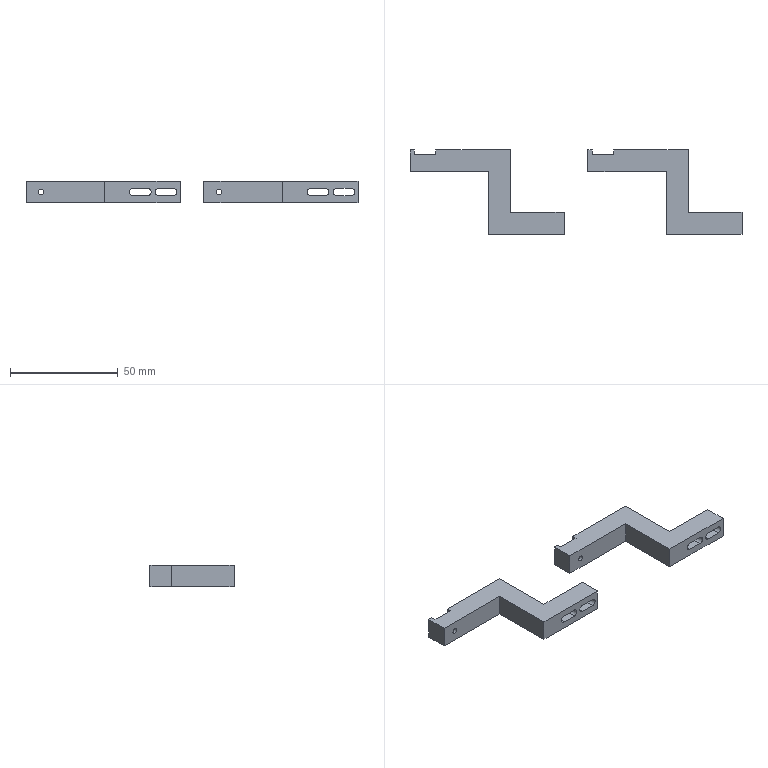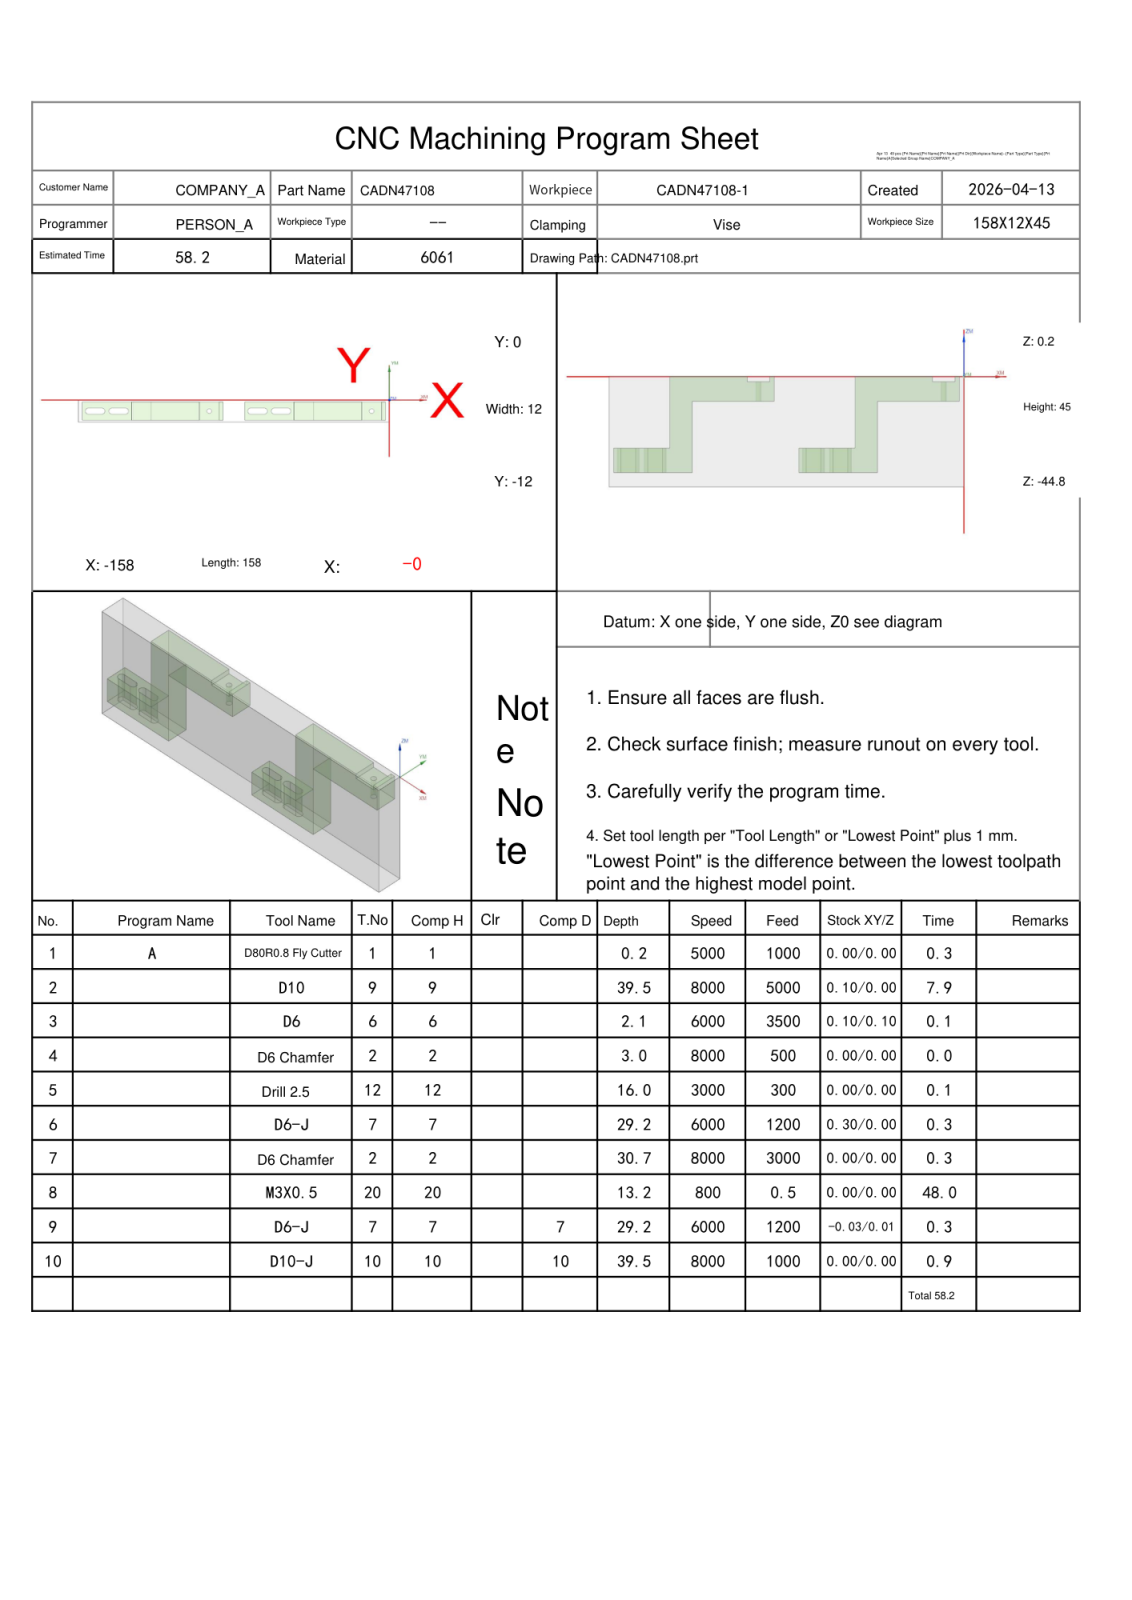NC program | NX | posted by the shop | part box 154 x 39 x 10 mm
Whole program, first 2157 of 3604 lines:
%
O0001
(Machine time: 104.10 MIN)
(===Total Tool:8===)
(T1=D80R0.8 Fly Cutter D=80.  R=0.8  D-  H01 Z=0.    )
(T9=D10     D=10.  R=0.   D-  H09 Z=-39.3 )
(T6=D6      D=6.   R=0.   D-  H06 Z=-1.9  )
(T2=D6 Chamfer   D=6.   R=0.   D-  H02 Z=-30.5 )
(T12=Drill 2.5  D=2.5  DR_a=118 D-  H12 Z=-15.75)
(T7=D6-J    D=6.   R=0.   D-  H07 Z=-29.  )
(T20=M3X0.5 D=2.5  DR_a=180 D-  H20 Z=-13.  )
(T10=D10-J  D=10.  R=0.   D10 H10 Z=-39.3 )
G80 G90 G17 G49 G40
G91 G28 Z0
M01
N1 T01 M06
(D80R0.8 Fly Cutter  D=80. R=0.8 H=01 ce=0.00 di=0.00)
G00 G90 G54 X-201. Y-6. M03 S5000
G43 H01 Z20.
M08
Z2.
G01 Z0.0 F1000.
X-196.
X38.
X43.
Z2.
G00 Z20.
G91 G28 Z0.0
M05
M09
G91 G28 Z0.0
M01
N2 T09 M06
(D10  D=10. R=0. H=09 ce=0.10 di=0.00)
G00 G90 G54 X-120.25 Y-16.1 M03 S8000
G43 H09 Z20.
M08
Z.5
G01 X-156. Z.354 F5000.
G02 X-161.1 Y-11. Z.321 I0.0 J5.1
G01 Y-1. Z.281
G02 X-156. Y4.1 Z.248 I5.1 J0.0
G01 X-84.5 Z-.044
G02 X-79.4 Y-1. Z-.077 I0.0 J-5.1
G01 Y-11. Z-.117
G02 X-84.5 Y-16.1 Z-.15 I-5.1 J0.0
G01 X-156. Z-.442
G02 X-161.1 Y-11. Z-.475 I0.0 J5.1
G01 Y-1. Z-.515
G02 X-156. Y4.1 Z-.548 I5.1 J0.0
G01 X-84.5 Z-.84
G02 X-79.4 Y-1. Z-.873 I0.0 J-5.1
G01 Y-11. Z-.913
G02 X-84.5 Y-16.1 Z-.946 I-5.1 J0.0
G01 X-156. Z-1.238
G02 X-161.1 Y-11. Z-1.271 I0.0 J5.1
G01 Y-1. Z-1.311
G02 X-156. Y4.1 Z-1.344 I5.1 J0.0
G01 X-84.5 Z-1.636
G02 X-79.4 Y-1. Z-1.669 I0.0 J-5.1
G01 Y-11. Z-1.709
G02 X-84.5 Y-16.1 Z-1.742 I-5.1 J0.0
G01 X-156. Z-2.034
G02 X-161.1 Y-11. Z-2.067 I0.0 J5.1
G01 Y-1. Z-2.107
G02 X-156. Y4.1 Z-2.14 I5.1 J0.0
G01 X-84.5 Z-2.432
G02 X-79.4 Y-1. Z-2.465 I0.0 J-5.1
G01 Y-11. Z-2.505
G02 X-84.5 Y-16.1 Z-2.538 I-5.1 J0.0
G01 X-156. Z-2.83
G02 X-161.1 Y-11. Z-2.863 I0.0 J5.1
G01 Y-1. Z-2.903
G02 X-156. Y4.1 Z-2.936 I5.1 J0.0
G01 X-84.5 Z-3.228
G02 X-79.4 Y-1. Z-3.261 I0.0 J-5.1
G01 Y-11. Z-3.301
G02 X-84.5 Y-16.1 Z-3.334 I-5.1 J0.0
G01 X-156. Z-3.626
G02 X-161.1 Y-11. Z-3.659 I0.0 J5.1
G01 Y-1. Z-3.699
G02 X-156. Y4.1 Z-3.732 I5.1 J0.0
G01 X-84.5 Z-4.024
G02 X-79.4 Y-1. Z-4.057 I0.0 J-5.1
G01 Y-11. Z-4.097
G02 X-84.5 Y-16.1 Z-4.13 I-5.1 J0.0
G01 X-156. Z-4.422
G02 X-161.1 Y-11. Z-4.455 I0.0 J5.1
G01 Y-1. Z-4.495
G02 X-156. Y4.1 Z-4.528 I5.1 J0.0
G01 X-84.5 Z-4.82
G02 X-79.4 Y-1. Z-4.853 I0.0 J-5.1
G01 Y-11. Z-4.893
G02 X-84.5 Y-16.1 Z-4.926 I-5.1 J0.0
G01 X-156. Z-5.218
G02 X-161.1 Y-11. Z-5.251 I0.0 J5.1
G01 Y-1. Z-5.291
G02 X-156. Y4.1 Z-5.324 I5.1 J0.0
G01 X-84.5 Z-5.616
G02 X-79.4 Y-1. Z-5.649 I0.0 J-5.1
G01 Y-11. Z-5.689
G02 X-84.5 Y-16.1 Z-5.722 I-5.1 J0.0
G01 X-156. Z-6.014
G02 X-161.1 Y-11. Z-6.047 I0.0 J5.1
G01 Y-1. Z-6.087
G02 X-156. Y4.1 Z-6.12 I5.1 J0.0
G01 X-84.5 Z-6.412
G02 X-79.4 Y-1. Z-6.445 I0.0 J-5.1
G01 Y-11. Z-6.485
G02 X-84.5 Y-16.1 Z-6.518 I-5.1 J0.0
G01 X-156. Z-6.81
G02 X-161.1 Y-11. Z-6.843 I0.0 J5.1
G01 Y-1. Z-6.883
G02 X-156. Y4.1 Z-6.916 I5.1 J0.0
G01 X-84.5 Z-7.208
G02 X-79.4 Y-1. Z-7.241 I0.0 J-5.1
G01 Y-11. Z-7.281
G02 X-84.5 Y-16.1 Z-7.314 I-5.1 J0.0
G01 X-156. Z-7.606
G02 X-161.1 Y-11. Z-7.639 I0.0 J5.1
G01 Y-1. Z-7.679
G02 X-156. Y4.1 Z-7.712 I5.1 J0.0
G01 X-84.5 Z-8.004
G02 X-79.4 Y-1. Z-8.037 I0.0 J-5.1
G01 Y-11. Z-8.077
G02 X-84.5 Y-16.1 Z-8.11 I-5.1 J0.0
G01 X-156. Z-8.402
G02 X-161.1 Y-11. Z-8.435 I0.0 J5.1
G01 Y-1. Z-8.475
G02 X-156. Y4.1 Z-8.508 I5.1 J0.0
G01 X-84.5 Z-8.8
G02 X-79.4 Y-1. Z-8.833 I0.0 J-5.1
G01 Y-11. Z-8.873
G02 X-84.5 Y-16.1 Z-8.906 I-5.1 J0.0
G01 X-156. Z-9.198
G02 X-161.1 Y-11. Z-9.231 I0.0 J5.1
G01 Y-1. Z-9.271
G02 X-156. Y4.1 Z-9.304 I5.1 J0.0
G01 X-84.5 Z-9.596
G02 X-79.4 Y-1. Z-9.629 I0.0 J-5.1
G01 Y-11. Z-9.669
G02 X-84.5 Y-16.1 Z-9.702 I-5.1 J0.0
G01 X-156. Z-9.994
G02 X-161.1 Y-11. Z-10.027 I0.0 J5.1
G01 Y-1. Z-10.067
G02 X-156. Y4.1 Z-10.1 I5.1 J0.0
G01 X-84.5 Z-10.392
G02 X-79.4 Y-1. Z-10.425 I0.0 J-5.1
G01 Y-11. Z-10.465
G02 X-84.5 Y-16.1 Z-10.498 I-5.1 J0.0
G01 X-156. Z-10.79
G02 X-161.1 Y-11. Z-10.823 I0.0 J5.1
G01 Y-1. Z-10.863
G02 X-156. Y4.1 Z-10.896 I5.1 J0.0
G01 X-84.5 Z-11.188
G02 X-79.4 Y-1. Z-11.221 I0.0 J-5.1
G01 Y-11. Z-11.261
G02 X-84.5 Y-16.1 Z-11.294 I-5.1 J0.0
G01 X-156. Z-11.586
G02 X-161.1 Y-11. Z-11.619 I0.0 J5.1
G01 Y-1. Z-11.659
G02 X-156. Y4.1 Z-11.692 I5.1 J0.0
G01 X-84.5 Z-11.984
G02 X-79.4 Y-1. Z-12.017 I0.0 J-5.1
G01 Y-11. Z-12.057
G02 X-84.5 Y-16.1 Z-12.09 I-5.1 J0.0
G01 X-156. Z-12.382
G02 X-161.1 Y-11. Z-12.415 I0.0 J5.1
G01 Y-1. Z-12.455
G02 X-156. Y4.1 Z-12.488 I5.1 J0.0
G01 X-84.5 Z-12.78
G02 X-79.4 Y-1. Z-12.813 I0.0 J-5.1
G01 Y-11. Z-12.853
G02 X-84.5 Y-16.1 Z-12.886 I-5.1 J0.0
G01 X-156. Z-13.178
G02 X-161.1 Y-11. Z-13.211 I0.0 J5.1
G01 Y-1. Z-13.251
G02 X-156. Y4.1 Z-13.284 I5.1 J0.0
G01 X-84.5 Z-13.576
G02 X-79.4 Y-1. Z-13.609 I0.0 J-5.1
G01 Y-11. Z-13.649
G02 X-84.5 Y-16.1 Z-13.682 I-5.1 J0.0
G01 X-156. Z-13.974
G02 X-161.1 Y-11. Z-14.007 I0.0 J5.1
G01 Y-1. Z-14.047
G02 X-156. Y4.1 Z-14.08 I5.1 J0.0
G01 X-84.5 Z-14.372
G02 X-79.4 Y-1. Z-14.405 I0.0 J-5.1
G01 Y-11. Z-14.445
G02 X-84.5 Y-16.1 Z-14.478 I-5.1 J0.0
G01 X-156. Z-14.77
G02 X-161.1 Y-11. Z-14.803 I0.0 J5.1
G01 Y-1. Z-14.843
G02 X-156. Y4.1 Z-14.876 I5.1 J0.0
G01 X-84.5 Z-15.168
G02 X-79.4 Y-1. Z-15.201 I0.0 J-5.1
G01 Y-11. Z-15.241
G02 X-84.5 Y-16.1 Z-15.274 I-5.1 J0.0
G01 X-156. Z-15.566
G02 X-161.1 Y-11. Z-15.599 I0.0 J5.1
G01 Y-1. Z-15.639
G02 X-156. Y4.1 Z-15.672 I5.1 J0.0
G01 X-84.5 Z-15.964
G02 X-79.4 Y-1. Z-15.997 I0.0 J-5.1
G01 Y-11. Z-16.037
G02 X-84.5 Y-16.1 Z-16.07 I-5.1 J0.0
G01 X-156. Z-16.362
G02 X-161.1 Y-11. Z-16.395 I0.0 J5.1
G01 Y-1. Z-16.435
G02 X-156. Y4.1 Z-16.468 I5.1 J0.0
G01 X-84.5 Z-16.76
G02 X-79.4 Y-1. Z-16.793 I0.0 J-5.1
G01 Y-11. Z-16.833
G02 X-84.5 Y-16.1 Z-16.866 I-5.1 J0.0
G01 X-156. Z-17.158
G02 X-161.1 Y-11. Z-17.191 I0.0 J5.1
G01 Y-1. Z-17.231
G02 X-156. Y4.1 Z-17.264 I5.1 J0.0
G01 X-84.5 Z-17.556
G02 X-79.4 Y-1. Z-17.589 I0.0 J-5.1
G01 Y-11. Z-17.629
G02 X-84.5 Y-16.1 Z-17.662 I-5.1 J0.0
G01 X-156. Z-17.954
G02 X-161.1 Y-11. Z-17.987 I0.0 J5.1
G01 Y-1. Z-18.027
G02 X-156. Y4.1 Z-18.06 I5.1 J0.0
G01 X-84.5 Z-18.352
G02 X-79.4 Y-1. Z-18.385 I0.0 J-5.1
G01 Y-11. Z-18.425
G02 X-84.5 Y-16.1 Z-18.458 I-5.1 J0.0
G01 X-156. Z-18.75
G02 X-161.1 Y-11. Z-18.783 I0.0 J5.1
G01 Y-1. Z-18.823
G02 X-156. Y4.1 Z-18.856 I5.1 J0.0
G01 X-84.5 Z-19.148
G02 X-79.4 Y-1. Z-19.181 I0.0 J-5.1
G01 Y-11. Z-19.221
G02 X-84.5 Y-16.1 Z-19.254 I-5.1 J0.0
G01 X-156. Z-19.546
G02 X-161.1 Y-11. Z-19.579 I0.0 J5.1
G01 Y-1. Z-19.619
G02 X-156. Y4.1 Z-19.652 I5.1 J0.0
G01 X-84.5 Z-19.944
G02 X-79.4 Y-1. Z-19.977 I0.0 J-5.1
G01 Y-11. Z-20.017
G02 X-84.5 Y-16.1 Z-20.05 I-5.1 J0.0
G01 X-156. Z-20.342
G02 X-161.1 Y-11. Z-20.375 I0.0 J5.1
G01 Y-1. Z-20.415
G02 X-156. Y4.1 Z-20.448 I5.1 J0.0
G01 X-84.5 Z-20.74
G02 X-79.4 Y-1. Z-20.773 I0.0 J-5.1
G01 Y-11. Z-20.813
G02 X-84.5 Y-16.1 Z-20.846 I-5.1 J0.0
G01 X-156. Z-21.138
G02 X-161.1 Y-11. Z-21.171 I0.0 J5.1
G01 Y-1. Z-21.211
G02 X-156. Y4.1 Z-21.244 I5.1 J0.0
G01 X-84.5 Z-21.536
G02 X-79.4 Y-1. Z-21.569 I0.0 J-5.1
G01 Y-11. Z-21.609
G02 X-84.5 Y-16.1 Z-21.642 I-5.1 J0.0
G01 X-156. Z-21.934
G02 X-161.1 Y-11. Z-21.967 I0.0 J5.1
G01 Y-1. Z-22.007
G02 X-156. Y4.1 Z-22.04 I5.1 J0.0
G01 X-84.5 Z-22.332
G02 X-79.4 Y-1. Z-22.365 I0.0 J-5.1
G01 Y-11. Z-22.405
G02 X-84.5 Y-16.1 Z-22.438 I-5.1 J0.0
G01 X-156. Z-22.73
G02 X-161.1 Y-11. Z-22.763 I0.0 J5.1
G01 Y-1. Z-22.803
G02 X-156. Y4.1 Z-22.836 I5.1 J0.0
G01 X-84.5 Z-23.128
G02 X-79.4 Y-1. Z-23.161 I0.0 J-5.1
G01 Y-11. Z-23.201
G02 X-84.5 Y-16.1 Z-23.234 I-5.1 J0.0
G01 X-156. Z-23.526
G02 X-161.1 Y-11. Z-23.559 I0.0 J5.1
G01 Y-1. Z-23.599
G02 X-156. Y4.1 Z-23.632 I5.1 J0.0
G01 X-84.5 Z-23.924
G02 X-79.4 Y-1. Z-23.957 I0.0 J-5.1
G01 Y-11. Z-23.997
G02 X-84.5 Y-16.1 Z-24.03 I-5.1 J0.0
G01 X-156. Z-24.322
G02 X-161.1 Y-11. Z-24.355 I0.0 J5.1
G01 Y-1. Z-24.395
G02 X-156. Y4.1 Z-24.428 I5.1 J0.0
G01 X-84.5 Z-24.72
G02 X-79.4 Y-1. Z-24.753 I0.0 J-5.1
G01 Y-11. Z-24.793
G02 X-84.5 Y-16.1 Z-24.826 I-5.1 J0.0
G01 X-156. Z-25.118
G02 X-161.1 Y-11. Z-25.151 I0.0 J5.1
G01 Y-1. Z-25.191
G02 X-156. Y4.1 Z-25.224 I5.1 J0.0
G01 X-84.5 Z-25.516
G02 X-79.4 Y-1. Z-25.549 I0.0 J-5.1
G01 Y-11. Z-25.589
G02 X-84.5 Y-16.1 Z-25.622 I-5.1 J0.0
G01 X-156. Z-25.914
G02 X-161.1 Y-11. Z-25.947 I0.0 J5.1
G01 Y-1. Z-25.987
G02 X-156. Y4.1 Z-26.02 I5.1 J0.0
G01 X-84.5 Z-26.312
G02 X-79.4 Y-1. Z-26.345 I0.0 J-5.1
G01 Y-11. Z-26.385
G02 X-84.5 Y-16.1 Z-26.418 I-5.1 J0.0
G01 X-156. Z-26.71
G02 X-161.1 Y-11. Z-26.743 I0.0 J5.1
G01 Y-1. Z-26.783
G02 X-156. Y4.1 Z-26.816 I5.1 J0.0
G01 X-84.5 Z-27.108
G02 X-79.4 Y-1. Z-27.141 I0.0 J-5.1
G01 Y-11. Z-27.181
G02 X-84.5 Y-16.1 Z-27.214 I-5.1 J0.0
G01 X-156. Z-27.506
G02 X-161.1 Y-11. Z-27.539 I0.0 J5.1
G01 Y-1. Z-27.579
G02 X-156. Y4.1 Z-27.612 I5.1 J0.0
G01 X-84.5 Z-27.904
G02 X-79.4 Y-1. Z-27.937 I0.0 J-5.1
G01 Y-11. Z-27.977
G02 X-84.5 Y-16.1 Z-28.01 I-5.1 J0.0
G01 X-156. Z-28.302
G02 X-161.1 Y-11. Z-28.335 I0.0 J5.1
G01 Y-1. Z-28.375
G02 X-156. Y4.1 Z-28.408 I5.1 J0.0
G01 X-84.5 Z-28.7
G02 X-79.4 Y-1. Z-28.733 I0.0 J-5.1
G01 Y-11. Z-28.773
G02 X-84.5 Y-16.1 Z-28.806 I-5.1 J0.0
G01 X-156. Z-29.098
G02 X-161.1 Y-11. Z-29.131 I0.0 J5.1
G01 Y-1. Z-29.171
G02 X-156. Y4.1 Z-29.204 I5.1 J0.0
G01 X-84.5 Z-29.496
G02 X-79.4 Y-1. Z-29.529 I0.0 J-5.1
G01 Y-11. Z-29.569
G02 X-84.5 Y-16.1 Z-29.602 I-5.1 J0.0
G01 X-156. Z-29.894
G02 X-161.1 Y-11. Z-29.927 I0.0 J5.1
G01 Y-1. Z-29.967
G02 X-156. Y4.1 Z-30. I5.1 J0.0
G01 X-84.5 Z-30.292
G02 X-79.4 Y-1. Z-30.325 I0.0 J-5.1
G01 Y-11. Z-30.365
G02 X-84.5 Y-16.1 Z-30.398 I-5.1 J0.0
G01 X-156. Z-30.69
G02 X-161.1 Y-11. Z-30.723 I0.0 J5.1
G01 Y-1. Z-30.763
G02 X-156. Y4.1 Z-30.796 I5.1 J0.0
G01 X-84.5 Z-31.088
G02 X-79.4 Y-1. Z-31.121 I0.0 J-5.1
G01 Y-11. Z-31.161
G02 X-84.5 Y-16.1 Z-31.194 I-5.1 J0.0
G01 X-156. Z-31.486
G02 X-161.1 Y-11. Z-31.519 I0.0 J5.1
G01 Y-1. Z-31.559
G02 X-156. Y4.1 Z-31.592 I5.1 J0.0
G01 X-84.5 Z-31.884
G02 X-79.4 Y-1. Z-31.917 I0.0 J-5.1
G01 Y-11. Z-31.957
G02 X-84.5 Y-16.1 Z-31.99 I-5.1 J0.0
G01 X-156. Z-32.282
G02 X-161.1 Y-11. Z-32.315 I0.0 J5.1
G01 Y-1. Z-32.355
G02 X-156. Y4.1 Z-32.388 I5.1 J0.0
G01 X-84.5 Z-32.68
G02 X-79.4 Y-1. Z-32.713 I0.0 J-5.1
G01 Y-11. Z-32.753
G02 X-84.5 Y-16.1 Z-32.786 I-5.1 J0.0
G01 X-156. Z-33.078
G02 X-161.1 Y-11. Z-33.111 I0.0 J5.1
G01 Y-1. Z-33.151
G02 X-156. Y4.1 Z-33.184 I5.1 J0.0
G01 X-84.5 Z-33.476
G02 X-79.4 Y-1. Z-33.509 I0.0 J-5.1
G01 Y-11. Z-33.549
G02 X-84.5 Y-16.1 Z-33.582 I-5.1 J0.0
G01 X-156. Z-33.874
G02 X-161.1 Y-11. Z-33.907 I0.0 J5.1
G01 Y-1. Z-33.947
G02 X-156. Y4.1 Z-33.98 I5.1 J0.0
G01 X-84.5 Z-34.272
G02 X-79.4 Y-1. Z-34.305 I0.0 J-5.1
G01 Y-11. Z-34.345
G02 X-84.5 Y-16.1 Z-34.378 I-5.1 J0.0
G01 X-156. Z-34.67
G02 X-161.1 Y-11. Z-34.703 I0.0 J5.1
G01 Y-1. Z-34.743
G02 X-156. Y4.1 Z-34.776 I5.1 J0.0
G01 X-84.5 Z-35.068
G02 X-79.4 Y-1. Z-35.101 I0.0 J-5.1
G01 Y-11. Z-35.141
G02 X-84.5 Y-16.1 Z-35.174 I-5.1 J0.0
G01 X-156. Z-35.466
G02 X-161.1 Y-11. Z-35.499 I0.0 J5.1
G01 Y-1. Z-35.539
G02 X-156. Y4.1 Z-35.572 I5.1 J0.0
G01 X-84.5 Z-35.864
G02 X-79.4 Y-1. Z-35.897 I0.0 J-5.1
G01 Y-11. Z-35.937
G02 X-84.5 Y-16.1 Z-35.97 I-5.1 J0.0
G01 X-156. Z-36.262
G02 X-161.1 Y-11. Z-36.295 I0.0 J5.1
G01 Y-1. Z-36.335
G02 X-156. Y4.1 Z-36.368 I5.1 J0.0
G01 X-84.5 Z-36.66
G02 X-79.4 Y-1. Z-36.693 I0.0 J-5.1
G01 Y-11. Z-36.733
G02 X-84.5 Y-16.1 Z-36.766 I-5.1 J0.0
G01 X-156. Z-37.058
G02 X-161.1 Y-11. Z-37.091 I0.0 J5.1
G01 Y-1. Z-37.131
G02 X-156. Y4.1 Z-37.164 I5.1 J0.0
G01 X-84.5 Z-37.456
G02 X-79.4 Y-1. Z-37.489 I0.0 J-5.1
G01 Y-11. Z-37.529
G02 X-84.5 Y-16.1 Z-37.562 I-5.1 J0.0
G01 X-156. Z-37.854
G02 X-161.1 Y-11. Z-37.887 I0.0 J5.1
G01 Y-1. Z-37.927
G02 X-156. Y4.1 Z-37.96 I5.1 J0.0
G01 X-84.5 Z-38.252
G02 X-79.4 Y-1. Z-38.285 I0.0 J-5.1
G01 Y-11. Z-38.325
G02 X-84.5 Y-16.1 Z-38.358 I-5.1 J0.0
G01 X-156. Z-38.65
G02 X-161.1 Y-11. Z-38.683 I0.0 J5.1
G01 Y-1. Z-38.723
G02 X-156. Y4.1 Z-38.756 I5.1 J0.0
G01 X-84.5 Z-39.048
G02 X-79.4 Y-1. Z-39.081 I0.0 J-5.1
G01 Y-11. Z-39.121
G02 X-84.5 Y-16.1 Z-39.154 I-5.1 J0.0
G01 X-120.25 Z-39.3
X-156.
G02 X-161.1 Y-11. I0.0 J5.1
G01 Y-1.
G02 X-156. Y4.1 I5.1 J0.0
G01 X-84.5
G02 X-79.4 Y-1. I0.0 J-5.1
G01 Y-11.
G02 X-84.5 Y-16.1 I-5.1 J0.0
G01 X-120.25
X-120.75
Z-38.3
G00 Z20.
X-37.75
Z.5
G01 X-73.5 Z.354
G02 X-78.6 Y-11. Z.321 I0.0 J5.1
G01 Y-1. Z.281
G02 X-73.5 Y4.1 Z.248 I5.1 J0.0
G01 X-2. Z-.044
G02 X3.1 Y-1. Z-.077 I0.0 J-5.1
G01 Y-11. Z-.117
G02 X-2. Y-16.1 Z-.15 I-5.1 J0.0
G01 X-73.5 Z-.442
G02 X-78.6 Y-11. Z-.475 I0.0 J5.1
G01 Y-1. Z-.515
G02 X-73.5 Y4.1 Z-.548 I5.1 J0.0
G01 X-2. Z-.84
G02 X3.1 Y-1. Z-.873 I0.0 J-5.1
G01 Y-11. Z-.913
G02 X-2. Y-16.1 Z-.946 I-5.1 J0.0
G01 X-73.5 Z-1.238
G02 X-78.6 Y-11. Z-1.271 I0.0 J5.1
G01 Y-1. Z-1.311
G02 X-73.5 Y4.1 Z-1.344 I5.1 J0.0
G01 X-2. Z-1.636
G02 X3.1 Y-1. Z-1.669 I0.0 J-5.1
G01 Y-11. Z-1.709
G02 X-2. Y-16.1 Z-1.742 I-5.1 J0.0
G01 X-73.5 Z-2.034
G02 X-78.6 Y-11. Z-2.067 I0.0 J5.1
G01 Y-1. Z-2.107
G02 X-73.5 Y4.1 Z-2.14 I5.1 J0.0
G01 X-2. Z-2.432
G02 X3.1 Y-1. Z-2.465 I0.0 J-5.1
G01 Y-11. Z-2.505
G02 X-2. Y-16.1 Z-2.538 I-5.1 J0.0
G01 X-73.5 Z-2.83
G02 X-78.6 Y-11. Z-2.863 I0.0 J5.1
G01 Y-1. Z-2.903
G02 X-73.5 Y4.1 Z-2.936 I5.1 J0.0
G01 X-2. Z-3.228
G02 X3.1 Y-1. Z-3.261 I0.0 J-5.1
G01 Y-11. Z-3.301
G02 X-2. Y-16.1 Z-3.334 I-5.1 J0.0
G01 X-73.5 Z-3.626
G02 X-78.6 Y-11. Z-3.659 I0.0 J5.1
G01 Y-1. Z-3.699
G02 X-73.5 Y4.1 Z-3.732 I5.1 J0.0
G01 X-2. Z-4.024
G02 X3.1 Y-1. Z-4.057 I0.0 J-5.1
G01 Y-11. Z-4.097
G02 X-2. Y-16.1 Z-4.13 I-5.1 J0.0
G01 X-73.5 Z-4.422
G02 X-78.6 Y-11. Z-4.455 I0.0 J5.1
G01 Y-1. Z-4.495
G02 X-73.5 Y4.1 Z-4.528 I5.1 J0.0
G01 X-2. Z-4.82
G02 X3.1 Y-1. Z-4.853 I0.0 J-5.1
G01 Y-11. Z-4.893
G02 X-2. Y-16.1 Z-4.926 I-5.1 J0.0
G01 X-73.5 Z-5.218
G02 X-78.6 Y-11. Z-5.251 I0.0 J5.1
G01 Y-1. Z-5.291
G02 X-73.5 Y4.1 Z-5.324 I5.1 J0.0
G01 X-2. Z-5.616
G02 X3.1 Y-1. Z-5.649 I0.0 J-5.1
G01 Y-11. Z-5.689
G02 X-2. Y-16.1 Z-5.722 I-5.1 J0.0
G01 X-73.5 Z-6.014
G02 X-78.6 Y-11. Z-6.047 I0.0 J5.1
G01 Y-1. Z-6.087
G02 X-73.5 Y4.1 Z-6.12 I5.1 J0.0
G01 X-2. Z-6.412
G02 X3.1 Y-1. Z-6.445 I0.0 J-5.1
G01 Y-11. Z-6.485
G02 X-2. Y-16.1 Z-6.518 I-5.1 J0.0
G01 X-73.5 Z-6.81
G02 X-78.6 Y-11. Z-6.843 I0.0 J5.1
G01 Y-1. Z-6.883
G02 X-73.5 Y4.1 Z-6.916 I5.1 J0.0
G01 X-2. Z-7.208
G02 X3.1 Y-1. Z-7.241 I0.0 J-5.1
G01 Y-11. Z-7.281
G02 X-2. Y-16.1 Z-7.314 I-5.1 J0.0
G01 X-73.5 Z-7.606
G02 X-78.6 Y-11. Z-7.639 I0.0 J5.1
G01 Y-1. Z-7.679
G02 X-73.5 Y4.1 Z-7.712 I5.1 J0.0
G01 X-2. Z-8.004
G02 X3.1 Y-1. Z-8.037 I0.0 J-5.1
G01 Y-11. Z-8.077
G02 X-2. Y-16.1 Z-8.11 I-5.1 J0.0
G01 X-73.5 Z-8.402
G02 X-78.6 Y-11. Z-8.435 I0.0 J5.1
G01 Y-1. Z-8.475
G02 X-73.5 Y4.1 Z-8.508 I5.1 J0.0
G01 X-2. Z-8.8
G02 X3.1 Y-1. Z-8.833 I0.0 J-5.1
G01 Y-11. Z-8.873
G02 X-2. Y-16.1 Z-8.906 I-5.1 J0.0
G01 X-73.5 Z-9.198
G02 X-78.6 Y-11. Z-9.231 I0.0 J5.1
G01 Y-1. Z-9.271
G02 X-73.5 Y4.1 Z-9.304 I5.1 J0.0
G01 X-2. Z-9.596
G02 X3.1 Y-1. Z-9.629 I0.0 J-5.1
G01 Y-11. Z-9.669
G02 X-2. Y-16.1 Z-9.702 I-5.1 J0.0
G01 X-73.5 Z-9.994
G02 X-78.6 Y-11. Z-10.027 I0.0 J5.1
G01 Y-1. Z-10.067
G02 X-73.5 Y4.1 Z-10.1 I5.1 J0.0
G01 X-2. Z-10.392
G02 X3.1 Y-1. Z-10.425 I0.0 J-5.1
G01 Y-11. Z-10.465
G02 X-2. Y-16.1 Z-10.498 I-5.1 J0.0
G01 X-73.5 Z-10.79
G02 X-78.6 Y-11. Z-10.823 I0.0 J5.1
G01 Y-1. Z-10.863
G02 X-73.5 Y4.1 Z-10.896 I5.1 J0.0
G01 X-2. Z-11.188
G02 X3.1 Y-1. Z-11.221 I0.0 J-5.1
G01 Y-11. Z-11.261
G02 X-2. Y-16.1 Z-11.294 I-5.1 J0.0
G01 X-73.5 Z-11.586
G02 X-78.6 Y-11. Z-11.619 I0.0 J5.1
G01 Y-1. Z-11.659
G02 X-73.5 Y4.1 Z-11.692 I5.1 J0.0
G01 X-2. Z-11.984
G02 X3.1 Y-1. Z-12.017 I0.0 J-5.1
G01 Y-11. Z-12.057
G02 X-2. Y-16.1 Z-12.09 I-5.1 J0.0
G01 X-73.5 Z-12.382
G02 X-78.6 Y-11. Z-12.415 I0.0 J5.1
G01 Y-1. Z-12.455
G02 X-73.5 Y4.1 Z-12.488 I5.1 J0.0
G01 X-2. Z-12.78
G02 X3.1 Y-1. Z-12.813 I0.0 J-5.1
G01 Y-11. Z-12.853
G02 X-2. Y-16.1 Z-12.886 I-5.1 J0.0
G01 X-73.5 Z-13.178
G02 X-78.6 Y-11. Z-13.211 I0.0 J5.1
G01 Y-1. Z-13.251
G02 X-73.5 Y4.1 Z-13.284 I5.1 J0.0
G01 X-2. Z-13.576
G02 X3.1 Y-1. Z-13.609 I0.0 J-5.1
G01 Y-11. Z-13.649
G02 X-2. Y-16.1 Z-13.682 I-5.1 J0.0
G01 X-73.5 Z-13.974
G02 X-78.6 Y-11. Z-14.007 I0.0 J5.1
G01 Y-1. Z-14.047
G02 X-73.5 Y4.1 Z-14.08 I5.1 J0.0
G01 X-2. Z-14.372
G02 X3.1 Y-1. Z-14.405 I0.0 J-5.1
G01 Y-11. Z-14.445
G02 X-2. Y-16.1 Z-14.478 I-5.1 J0.0
G01 X-73.5 Z-14.77
G02 X-78.6 Y-11. Z-14.803 I0.0 J5.1
G01 Y-1. Z-14.843
G02 X-73.5 Y4.1 Z-14.876 I5.1 J0.0
G01 X-2. Z-15.168
G02 X3.1 Y-1. Z-15.201 I0.0 J-5.1
G01 Y-11. Z-15.241
G02 X-2. Y-16.1 Z-15.274 I-5.1 J0.0
G01 X-73.5 Z-15.566
G02 X-78.6 Y-11. Z-15.599 I0.0 J5.1
G01 Y-1. Z-15.639
G02 X-73.5 Y4.1 Z-15.672 I5.1 J0.0
G01 X-2. Z-15.964
G02 X3.1 Y-1. Z-15.997 I0.0 J-5.1
G01 Y-11. Z-16.037
G02 X-2. Y-16.1 Z-16.07 I-5.1 J0.0
G01 X-73.5 Z-16.362
G02 X-78.6 Y-11. Z-16.395 I0.0 J5.1
G01 Y-1. Z-16.435
G02 X-73.5 Y4.1 Z-16.468 I5.1 J0.0
G01 X-2. Z-16.76
G02 X3.1 Y-1. Z-16.793 I0.0 J-5.1
G01 Y-11. Z-16.833
G02 X-2. Y-16.1 Z-16.866 I-5.1 J0.0
G01 X-73.5 Z-17.158
G02 X-78.6 Y-11. Z-17.191 I0.0 J5.1
G01 Y-1. Z-17.231
G02 X-73.5 Y4.1 Z-17.264 I5.1 J0.0
G01 X-2. Z-17.556
G02 X3.1 Y-1. Z-17.589 I0.0 J-5.1
G01 Y-11. Z-17.629
G02 X-2. Y-16.1 Z-17.662 I-5.1 J0.0
G01 X-73.5 Z-17.954
G02 X-78.6 Y-11. Z-17.987 I0.0 J5.1
G01 Y-1. Z-18.027
G02 X-73.5 Y4.1 Z-18.06 I5.1 J0.0
G01 X-2. Z-18.352
G02 X3.1 Y-1. Z-18.385 I0.0 J-5.1
G01 Y-11. Z-18.425
G02 X-2. Y-16.1 Z-18.458 I-5.1 J0.0
G01 X-73.5 Z-18.75
G02 X-78.6 Y-11. Z-18.783 I0.0 J5.1
G01 Y-1. Z-18.823
G02 X-73.5 Y4.1 Z-18.856 I5.1 J0.0
G01 X-2. Z-19.148
G02 X3.1 Y-1. Z-19.181 I0.0 J-5.1
G01 Y-11. Z-19.221
G02 X-2. Y-16.1 Z-19.254 I-5.1 J0.0
G01 X-73.5 Z-19.546
G02 X-78.6 Y-11. Z-19.579 I0.0 J5.1
G01 Y-1. Z-19.619
G02 X-73.5 Y4.1 Z-19.652 I5.1 J0.0
G01 X-2. Z-19.944
G02 X3.1 Y-1. Z-19.977 I0.0 J-5.1
G01 Y-11. Z-20.017
G02 X-2. Y-16.1 Z-20.05 I-5.1 J0.0
G01 X-73.5 Z-20.342
G02 X-78.6 Y-11. Z-20.375 I0.0 J5.1
G01 Y-1. Z-20.415
G02 X-73.5 Y4.1 Z-20.448 I5.1 J0.0
G01 X-2. Z-20.74
G02 X3.1 Y-1. Z-20.773 I0.0 J-5.1
G01 Y-11. Z-20.813
G02 X-2. Y-16.1 Z-20.846 I-5.1 J0.0
G01 X-73.5 Z-21.138
G02 X-78.6 Y-11. Z-21.171 I0.0 J5.1
G01 Y-1. Z-21.211
G02 X-73.5 Y4.1 Z-21.244 I5.1 J0.0
G01 X-2. Z-21.536
G02 X3.1 Y-1. Z-21.569 I0.0 J-5.1
G01 Y-11. Z-21.609
G02 X-2. Y-16.1 Z-21.642 I-5.1 J0.0
G01 X-73.5 Z-21.934
G02 X-78.6 Y-11. Z-21.967 I0.0 J5.1
G01 Y-1. Z-22.007
G02 X-73.5 Y4.1 Z-22.04 I5.1 J0.0
G01 X-2. Z-22.332
G02 X3.1 Y-1. Z-22.365 I0.0 J-5.1
G01 Y-11. Z-22.405
G02 X-2. Y-16.1 Z-22.438 I-5.1 J0.0
G01 X-73.5 Z-22.73
G02 X-78.6 Y-11. Z-22.763 I0.0 J5.1
G01 Y-1. Z-22.803
G02 X-73.5 Y4.1 Z-22.836 I5.1 J0.0
G01 X-2. Z-23.128
G02 X3.1 Y-1. Z-23.161 I0.0 J-5.1
G01 Y-11. Z-23.201
G02 X-2. Y-16.1 Z-23.234 I-5.1 J0.0
G01 X-73.5 Z-23.526
G02 X-78.6 Y-11. Z-23.559 I0.0 J5.1
G01 Y-1. Z-23.599
G02 X-73.5 Y4.1 Z-23.632 I5.1 J0.0
G01 X-2. Z-23.924
G02 X3.1 Y-1. Z-23.957 I0.0 J-5.1
G01 Y-11. Z-23.997
G02 X-2. Y-16.1 Z-24.03 I-5.1 J0.0
G01 X-73.5 Z-24.322
G02 X-78.6 Y-11. Z-24.355 I0.0 J5.1
G01 Y-1. Z-24.395
G02 X-73.5 Y4.1 Z-24.428 I5.1 J0.0
G01 X-2. Z-24.72
G02 X3.1 Y-1. Z-24.753 I0.0 J-5.1
G01 Y-11. Z-24.793
G02 X-2. Y-16.1 Z-24.826 I-5.1 J0.0
G01 X-73.5 Z-25.118
G02 X-78.6 Y-11. Z-25.151 I0.0 J5.1
G01 Y-1. Z-25.191
G02 X-73.5 Y4.1 Z-25.224 I5.1 J0.0
G01 X-2. Z-25.516
G02 X3.1 Y-1. Z-25.549 I0.0 J-5.1
G01 Y-11. Z-25.589
G02 X-2. Y-16.1 Z-25.622 I-5.1 J0.0
G01 X-73.5 Z-25.914
G02 X-78.6 Y-11. Z-25.947 I0.0 J5.1
G01 Y-1. Z-25.987
G02 X-73.5 Y4.1 Z-26.02 I5.1 J0.0
G01 X-2. Z-26.312
G02 X3.1 Y-1. Z-26.345 I0.0 J-5.1
G01 Y-11. Z-26.385
G02 X-2. Y-16.1 Z-26.418 I-5.1 J0.0
G01 X-73.5 Z-26.71
G02 X-78.6 Y-11. Z-26.743 I0.0 J5.1
G01 Y-1. Z-26.783
G02 X-73.5 Y4.1 Z-26.816 I5.1 J0.0
G01 X-2. Z-27.108
G02 X3.1 Y-1. Z-27.141 I0.0 J-5.1
G01 Y-11. Z-27.181
G02 X-2. Y-16.1 Z-27.214 I-5.1 J0.0
G01 X-73.5 Z-27.506
G02 X-78.6 Y-11. Z-27.539 I0.0 J5.1
G01 Y-1. Z-27.579
G02 X-73.5 Y4.1 Z-27.612 I5.1 J0.0
G01 X-2. Z-27.904
G02 X3.1 Y-1. Z-27.937 I0.0 J-5.1
G01 Y-11. Z-27.977
G02 X-2. Y-16.1 Z-28.01 I-5.1 J0.0
G01 X-73.5 Z-28.302
G02 X-78.6 Y-11. Z-28.335 I0.0 J5.1
G01 Y-1. Z-28.375
G02 X-73.5 Y4.1 Z-28.408 I5.1 J0.0
G01 X-2. Z-28.7
G02 X3.1 Y-1. Z-28.733 I0.0 J-5.1
G01 Y-11. Z-28.773
G02 X-2. Y-16.1 Z-28.806 I-5.1 J0.0
G01 X-73.5 Z-29.098
G02 X-78.6 Y-11. Z-29.131 I0.0 J5.1
G01 Y-1. Z-29.171
G02 X-73.5 Y4.1 Z-29.204 I5.1 J0.0
G01 X-2. Z-29.496
G02 X3.1 Y-1. Z-29.529 I0.0 J-5.1
G01 Y-11. Z-29.569
G02 X-2. Y-16.1 Z-29.602 I-5.1 J0.0
G01 X-73.5 Z-29.894
G02 X-78.6 Y-11. Z-29.927 I0.0 J5.1
G01 Y-1. Z-29.967
G02 X-73.5 Y4.1 Z-30. I5.1 J0.0
G01 X-2. Z-30.292
G02 X3.1 Y-1. Z-30.325 I0.0 J-5.1
G01 Y-11. Z-30.365
G02 X-2. Y-16.1 Z-30.398 I-5.1 J0.0
G01 X-73.5 Z-30.69
G02 X-78.6 Y-11. Z-30.723 I0.0 J5.1
G01 Y-1. Z-30.763
G02 X-73.5 Y4.1 Z-30.796 I5.1 J0.0
G01 X-2. Z-31.088
G02 X3.1 Y-1. Z-31.121 I0.0 J-5.1
G01 Y-11. Z-31.161
G02 X-2. Y-16.1 Z-31.194 I-5.1 J0.0
G01 X-73.5 Z-31.486
G02 X-78.6 Y-11. Z-31.519 I0.0 J5.1
G01 Y-1. Z-31.559
G02 X-73.5 Y4.1 Z-31.592 I5.1 J0.0
G01 X-2. Z-31.884
G02 X3.1 Y-1. Z-31.917 I0.0 J-5.1
G01 Y-11. Z-31.957
G02 X-2. Y-16.1 Z-31.99 I-5.1 J0.0
G01 X-73.5 Z-32.282
G02 X-78.6 Y-11. Z-32.315 I0.0 J5.1
G01 Y-1. Z-32.355
G02 X-73.5 Y4.1 Z-32.388 I5.1 J0.0
G01 X-2. Z-32.68
G02 X3.1 Y-1. Z-32.713 I0.0 J-5.1
G01 Y-11. Z-32.753
G02 X-2. Y-16.1 Z-32.786 I-5.1 J0.0
G01 X-73.5 Z-33.078
G02 X-78.6 Y-11. Z-33.111 I0.0 J5.1
G01 Y-1. Z-33.151
G02 X-73.5 Y4.1 Z-33.184 I5.1 J0.0
G01 X-2. Z-33.476
G02 X3.1 Y-1. Z-33.509 I0.0 J-5.1
G01 Y-11. Z-33.549
G02 X-2. Y-16.1 Z-33.582 I-5.1 J0.0
G01 X-73.5 Z-33.874
G02 X-78.6 Y-11. Z-33.907 I0.0 J5.1
G01 Y-1. Z-33.947
G02 X-73.5 Y4.1 Z-33.98 I5.1 J0.0
G01 X-2. Z-34.272
G02 X3.1 Y-1. Z-34.305 I0.0 J-5.1
G01 Y-11. Z-34.345
G02 X-2. Y-16.1 Z-34.378 I-5.1 J0.0
G01 X-73.5 Z-34.67
G02 X-78.6 Y-11. Z-34.703 I0.0 J5.1
G01 Y-1. Z-34.743
G02 X-73.5 Y4.1 Z-34.776 I5.1 J0.0
G01 X-2. Z-35.068
G02 X3.1 Y-1. Z-35.101 I0.0 J-5.1
G01 Y-11. Z-35.141
G02 X-2. Y-16.1 Z-35.174 I-5.1 J0.0
G01 X-73.5 Z-35.466
G02 X-78.6 Y-11. Z-35.499 I0.0 J5.1
G01 Y-1. Z-35.539
G02 X-73.5 Y4.1 Z-35.572 I5.1 J0.0
G01 X-2. Z-35.864
G02 X3.1 Y-1. Z-35.897 I0.0 J-5.1
G01 Y-11. Z-35.937
G02 X-2. Y-16.1 Z-35.97 I-5.1 J0.0
G01 X-73.5 Z-36.262
G02 X-78.6 Y-11. Z-36.295 I0.0 J5.1
G01 Y-1. Z-36.335
G02 X-73.5 Y4.1 Z-36.368 I5.1 J0.0
G01 X-2. Z-36.66
G02 X3.1 Y-1. Z-36.693 I0.0 J-5.1
G01 Y-11. Z-36.733
G02 X-2. Y-16.1 Z-36.766 I-5.1 J0.0
G01 X-73.5 Z-37.058
G02 X-78.6 Y-11. Z-37.091 I0.0 J5.1
G01 Y-1. Z-37.131
G02 X-73.5 Y4.1 Z-37.164 I5.1 J0.0
G01 X-2. Z-37.456
G02 X3.1 Y-1. Z-37.489 I0.0 J-5.1
G01 Y-11. Z-37.529
G02 X-2. Y-16.1 Z-37.562 I-5.1 J0.0
G01 X-73.5 Z-37.854
G02 X-78.6 Y-11. Z-37.887 I0.0 J5.1
G01 Y-1. Z-37.927
G02 X-73.5 Y4.1 Z-37.96 I5.1 J0.0
G01 X-2. Z-38.252
G02 X3.1 Y-1. Z-38.285 I0.0 J-5.1
G01 Y-11. Z-38.325
G02 X-2. Y-16.1 Z-38.358 I-5.1 J0.0
G01 X-73.5 Z-38.65
G02 X-78.6 Y-11. Z-38.683 I0.0 J5.1
G01 Y-1. Z-38.723
G02 X-73.5 Y4.1 Z-38.756 I5.1 J0.0
G01 X-2. Z-39.048
G02 X3.1 Y-1. Z-39.081 I0.0 J-5.1
G01 Y-11. Z-39.121
G02 X-2. Y-16.1 Z-39.154 I-5.1 J0.0
G01 X-37.75 Z-39.3
X-73.5
G02 X-78.6 Y-11. I0.0 J5.1
G01 Y-1.
G02 X-73.5 Y4.1 I5.1 J0.0
G01 X-2.
G02 X3.1 Y-1. I0.0 J-5.1
G01 Y-11.
G02 X-2. Y-16.1 I-5.1 J0.0
G01 X-37.75
X-38.25
Z-38.3
G00 Z20.
G00 G90 X-146.55 Y7. M03 S6000
Z20.
Z.002
G01 Z-.498 F3500.
Y-4.5
X-152.5
Y-7.5
X-140.6
Y-4.5
X-146.55
Y0.0
X-157.
Y-12.
X-136.1
Y0.0
X-146.55
X-147.05
Z.002
G00 Z.5
X-146.55 Y7.
Z-.497
G01 Z-.997
Y-4.5
X-152.5
Y-7.5
X-140.6
Y-4.5
X-146.55
Y0.0
X-157.
Y-12.
X-136.1
Y0.0
X-146.55
X-147.05
Z-.497
G00 Z.002
X-146.55 Y7.
Z-.995
G01 Z-1.495
Y-4.5
X-152.5
Y-7.5
X-140.6
Y-4.5
X-146.55
Y0.0
X-157.
Y-12.
X-136.1
Y0.0
X-146.55
X-147.05
Z-.995
G00 Z-.497
X-146.55 Y7.
Z-1.493
G01 Z-1.993
Y-4.5
X-152.5
Y-7.5
X-140.6
Y-4.5
X-146.55
Y0.0
X-157.
Y-12.
X-136.1
Y0.0
X-146.55
X-147.05
Z-1.493
G00 Z-.995
X-146.55 Y7.
Z-1.991
G01 Z-2.491
Y-4.5
X-152.5
Y-7.5
X-140.6
Y-4.5
X-146.55
Y0.0
X-157.
Y-12.
X-136.1
Y0.0
X-146.55
X-147.05
Z-1.991
G00 Z-1.493
X-146.55 Y7.
Z-2.49
G01 Z-2.99
Y-4.5
X-152.5
Y-7.5
X-140.6
Y-4.5
X-146.55
Y0.0
X-157.
Y-12.
X-136.1
Y0.0
X-146.55
X-147.05
Z-2.49
G00 Z-1.991
X-146.55 Y7.
Z-2.988
G01 Z-3.488
Y-4.5
X-152.5
Y-7.5
X-140.6
Y-4.5
X-146.55
Y0.0
X-157.
Y-12.
X-136.1
Y0.0
X-146.55
X-147.05
Z-2.988
G00 Z-2.49
X-146.55 Y7.
Z-3.486
G01 Z-3.986
Y-4.5
X-152.5
Y-7.5
X-140.6
Y-4.5
X-146.55
Y0.0
X-157.
Y-12.
X-136.1
Y0.0
X-146.55
X-147.05
Z-3.486
G00 Z-2.988
X-146.55 Y7.
Z-3.984
G01 Z-4.484
Y-4.5
X-152.5
Y-7.5
X-140.6
Y-4.5
X-146.55
Y0.0
X-157.
Y-12.
X-136.1
Y0.0
X-146.55
X-147.05
Z-3.984
G00 Z-3.486
X-146.55 Y7.
Z-4.483
G01 Z-4.983
Y-4.5
X-152.5
Y-7.5
X-140.6
Y-4.5
X-146.55
Y0.0
X-157.
Y-12.
X-136.1
Y0.0
X-146.55
X-147.05
Z-4.483
G00 Z-3.984
X-146.55 Y7.
Z-4.981
G01 Z-5.481
Y-4.5
X-152.5
Y-7.5
X-140.6
Y-4.5
X-146.55
Y0.0
X-157.
Y-12.
X-136.1
Y0.0
X-146.55
X-147.05
Z-4.981
G00 Z-4.483
X-146.55 Y7.
Z-5.479
G01 Z-5.979
Y-4.5
X-152.5
Y-7.5
X-140.6
Y-4.5
X-146.55
Y0.0
X-157.
Y-12.
X-136.1
Y0.0
X-146.55
X-147.05
Z-5.479
G00 Z-4.981
X-146.55 Y7.
Z-5.978
G01 Z-6.478
Y-4.5
X-152.5
Y-7.5
X-140.6
Y-4.5
X-146.55
Y0.0
X-157.
Y-12.
X-136.1
Y0.0
X-146.55
X-147.05
Z-5.978
G00 Z-5.479
X-146.55 Y7.
Z-6.476
G01 Z-6.976
Y-4.5
X-152.5
Y-7.5
X-140.6
Y-4.5
X-146.55
Y0.0
X-157.
Y-12.
X-136.1
Y0.0
X-146.55
X-147.05
Z-6.476
G00 Z-5.978
X-146.55 Y7.
Z-6.974
G01 Z-7.474
Y-4.5
X-152.5
Y-7.5
X-140.6
Y-4.5
X-146.55
Y0.0
X-157.
Y-12.
X-136.1
Y0.0
X-146.55
X-147.05
Z-6.974
G00 Z-6.476
X-146.55 Y7.
Z-7.472
G01 Z-7.972
Y-4.5
X-152.5
Y-7.5
X-140.6
Y-4.5
X-146.55
Y0.0
X-157.
Y-12.
X-136.1
Y0.0
X-146.55
X-147.05
Z-7.472
G00 Z-6.974
X-146.55 Y7.
Z-7.971
G01 Z-8.471
Y-4.5
X-152.5
Y-7.5
X-140.6
Y-4.5
X-146.55
Y0.0
X-157.
Y-12.
X-136.1
Y0.0
X-146.55
X-147.05
Z-7.971
G00 Z-7.472
X-146.55 Y7.
Z-8.469
G01 Z-8.969
Y-4.5
X-152.5
Y-7.5
X-140.6
Y-4.5
X-146.55
Y0.0
X-157.
Y-12.
X-136.1
Y0.0
X-146.55
X-147.05
Z-8.469
G00 Z-7.971
X-146.55 Y7.
Z-8.967
G01 Z-9.467
Y-4.5
X-152.5
Y-7.5
X-140.6
Y-4.5
X-146.55
Y0.0
X-157.
Y-12.
X-136.1
Y0.0
X-146.55
X-147.05
Z-8.967
G00 Z-8.469
X-146.55 Y7.
Z-9.466
G01 Z-9.966
Y-4.5
X-152.5
Y-7.5
X-140.6
Y-4.5
X-146.55
Y0.0
X-157.
Y-12.
X-136.1
Y0.0
X-146.55
X-147.05
Z-9.466
G00 Z-8.967
X-146.55 Y7.
Z-9.964
G01 Z-10.464
Y-4.5
X-152.5
Y-7.5
X-140.6
Y-4.5
X-146.55
Y0.0
X-157.
Y-12.
X-136.1
Y0.0
X-146.55
X-147.05
Z-9.964
G00 Z-9.466
X-146.55 Y7.
Z-10.462
G01 Z-10.962
Y-4.5
X-152.5
Y-7.5
X-140.6
Y-4.5
X-146.55
Y0.0
X-157.
Y-12.
X-136.1
Y0.0
X-146.55
X-147.05
Z-10.462
G00 Z-9.964
X-146.55 Y7.
Z-10.96
G01 Z-11.46
Y-4.5
X-152.5
Y-7.5
X-140.6
Y-4.5
X-146.55
Y0.0
X-157.
Y-12.
X-136.1
Y0.0
X-146.55
X-147.05
Z-10.96
G00 Z-10.462
X-146.55 Y7.
Z-11.459
G01 Z-11.959
Y-4.5
X-152.5
Y-7.5
X-140.6
Y-4.5
X-146.55
Y0.0
X-157.
Y-12.
X-136.1
Y0.0
X-146.55
X-147.05
Z-11.459
G00 Z-10.96
X-146.55 Y7.
Z-11.957
G01 Z-12.457
Y-4.5
X-152.5
Y-7.5
X-140.6
Y-4.5
X-146.55
Y0.0
X-157.
Y-12.
X-136.1
Y0.0
X-146.55
X-147.05
Z-11.957
G00 Z-11.459
X-146.55 Y7.
Z-12.455
G01 Z-12.955
Y-4.5
X-152.5
Y-7.5
X-140.6
Y-4.5
X-146.55
Y0.0
X-157.
Y-12.
X-136.1
Y0.0
X-146.55
X-147.05
Z-12.455
G00 Z-11.957
X-146.55 Y7.
Z-12.953
G01 Z-13.453
Y-4.5
X-152.5
Y-7.5
X-140.6
Y-4.5
X-146.55
Y0.0
X-157.
Y-12.
X-136.1
Y0.0
X-146.55
X-147.05
Z-12.953
G00 Z-12.455
X-146.55 Y7.
Z-13.452
G01 Z-13.952
Y-4.5
X-152.5
Y-7.5
X-140.6
Y-4.5
X-146.55
Y0.0
X-157.
Y-12.
X-136.1
Y0.0
X-146.55
X-147.05
Z-13.452
G00 Z-12.953
X-146.55 Y7.
Z-13.95
G01 Z-14.45
Y-4.5
X-152.5
Y-7.5
X-140.6
Y-4.5
X-146.55
Y0.0
X-157.
Y-12.
X-136.1
Y0.0
X-146.55
X-147.05
Z-13.95
G00 Z-13.452
X-146.55 Y7.
Z-14.448
G01 Z-14.948
Y-4.5
X-152.5
Y-7.5
X-140.6
Y-4.5
X-146.55
Y0.0
X-157.
Y-12.
X-136.1
Y0.0
X-146.55
X-147.05
Z-14.448
G00 Z-13.95
X-146.55 Y7.
Z-14.947
G01 Z-15.447
Y-4.5
X-152.5
Y-7.5
X-140.6
Y-4.5
X-146.55
Y0.0
X-157.
Y-12.
X-136.1
Y0.0
X-146.55
X-147.05
Z-14.947
G00 Z-14.448
X-146.55 Y7.
Z-15.445
G01 Z-15.945
Y-4.5
X-152.5
Y-7.5
X-140.6
Y-4.5
X-146.55
Y0.0
X-157.
Y-12.
X-136.1
Y0.0
X-146.55
X-147.05
Z-15.445
G00 Z-14.947
X-146.55 Y7.
Z-15.943
G01 Z-16.443
Y-4.5
X-152.5
Y-7.5
X-140.6
Y-4.5
X-146.55
Y0.0
X-157.
Y-12.
X-136.1
Y0.0
X-146.55
X-147.05
Z-15.943
G00 Z-15.445
X-146.55 Y7.
Z-16.441
G01 Z-16.941
Y-4.5
X-152.5
Y-7.5
X-140.6
Y-4.5
X-146.55
Y0.0
X-157.
Y-12.
X-136.1
Y0.0
X-146.55
X-147.05
Z-16.441
G00 Z-15.943
X-146.55 Y7.
Z-16.94
G01 Z-17.44
Y-4.5
X-152.5
Y-7.5
X-140.6
Y-4.5
X-146.55
Y0.0
X-157.
Y-12.
X-136.1
Y0.0
X-146.55
X-147.05
Z-16.94
G00 Z-16.441
X-146.55 Y7.
Z-17.438
G01 Z-17.938
Y-4.5
X-152.5
Y-7.5
X-140.6
Y-4.5
X-146.55
Y0.0
X-157.
Y-12.
X-136.1
Y0.0
X-146.55
X-147.05
Z-17.438
G00 Z-16.94
X-146.55 Y7.
Z-17.936
G01 Z-18.436
Y-4.5
X-152.5
Y-7.5
X-140.6
Y-4.5
X-146.55
Y0.0
X-157.
Y-12.
X-136.1
Y0.0
X-146.55
X-147.05
Z-17.936
G00 Z-17.438
X-146.55 Y7.
Z-18.434
G01 Z-18.934
Y-4.5
X-152.5
Y-7.5
X-140.6
Y-4.5
X-146.55
Y0.0
X-157.
Y-12.
X-136.1
Y0.0
X-146.55
X-147.05
Z-18.434
G00 Z-17.936
X-146.55 Y7.
Z-18.933
G01 Z-19.433
Y-4.5
X-152.5
Y-7.5
X-140.6
Y-4.5
X-146.55
Y0.0
X-157.
Y-12.
X-136.1
Y0.0
X-146.55
X-147.05
Z-18.933
G00 Z-18.434
X-146.55 Y7.
Z-19.431
G01 Z-19.931
Y-4.5
X-152.5
Y-7.5
X-140.6
Y-4.5
X-146.55
Y0.0
X-157.
Y-12.
X-136.1
Y0.0
X-146.55
X-147.05
Z-19.431
G00 Z-18.933
X-146.55 Y7.
Z-19.929
G01 Z-20.429
Y-4.5
X-152.5
Y-7.5
X-140.6
Y-4.5
X-146.55
Y0.0
X-157.
Y-12.
X-136.1
Y0.0
X-146.55
X-147.05
Z-19.929
G00 Z-19.431
X-146.55 Y7.
Z-20.428
G01 Z-20.928
Y-4.5
X-152.5
Y-7.5
X-140.6
Y-4.5
X-146.55
Y0.0
X-157.
Y-12.
X-136.1
Y0.0
X-146.55
X-147.05
Z-20.428
G00 Z-19.929
X-146.55 Y7.
Z-20.926
G01 Z-21.426
Y-4.5
X-152.5
Y-7.5
X-140.6
Y-4.5
X-146.55
Y0.0
X-157.
Y-12.
X-136.1
Y0.0
X-146.55
X-147.05
Z-20.926
G00 Z-20.428
X-146.55 Y7.
Z-21.424
G01 Z-21.924
Y-4.5
X-152.5
Y-7.5
X-140.6
Y-4.5
X-146.55
Y0.0
X-157.
Y-12.
X-136.1
Y0.0
X-146.55
X-147.05
Z-21.424
G00 Z-20.926
X-146.55 Y7.
Z-21.922
G01 Z-22.422
Y-4.5
X-152.5
Y-7.5
X-140.6
Y-4.5
X-146.55
Y0.0
X-157.
Y-12.
X-136.1
Y0.0
X-146.55
X-147.05
Z-21.922
G00 Z-21.424
X-146.55 Y7.
Z-22.421
G01 Z-22.921
Y-4.5
X-152.5
Y-7.5
X-140.6
Y-4.5
X-146.55
Y0.0
X-157.
Y-12.
X-136.1
Y0.0
X-146.55
X-147.05
Z-22.421
G00 Z-21.922
X-146.55 Y7.
Z-22.919
G01 Z-23.419
Y-4.5
X-152.5
Y-7.5
X-140.6
Y-4.5
X-146.55
Y0.0
X-157.
Y-12.
X-136.1
Y0.0
X-146.55
X-147.05
Z-22.919
G00 Z-22.421
X-146.55 Y7.
Z-23.417
G01 Z-23.917
Y-4.5
X-152.5
Y-7.5
X-140.6
Y-4.5
X-146.55
Y0.0
X-157.
Y-12.
X-136.1
Y0.0
X-146.55
X-147.05
Z-23.417
G00 Z-22.919
X-146.55 Y7.
Z-23.916
G01 Z-24.416
Y-4.5
X-152.5
Y-7.5
X-140.6
Y-4.5
X-146.55
Y0.0
X-157.
Y-12.
X-136.1
Y0.0
X-146.55
X-147.05
Z-23.916
G00 Z-23.417
X-146.55 Y7.
Z-24.414
G01 Z-24.914
Y-4.5
X-152.5
Y-7.5
X-140.6
Y-4.5
X-146.55
Y0.0
X-157.
Y-12.
X-136.1
Y0.0
X-146.55
X-147.05
Z-24.414
G00 Z-23.916
X-146.55 Y7.
Z-24.912
G01 Z-25.412
Y-4.5
X-152.5
Y-7.5
X-140.6
Y-4.5
X-146.55
Y0.0
X-157.
Y-12.
X-136.1
Y0.0
X-146.55
X-147.05
Z-24.912
G00 Z-24.414
X-146.55 Y7.
Z-25.41
G01 Z-25.91
Y-4.5
X-152.5
Y-7.5
X-140.6
Y-4.5
X-146.55
Y0.0
X-157.
Y-12.
X-136.1
Y0.0
X-146.55
X-147.05
Z-25.41
G00 Z-24.912
X-146.55 Y7.
Z-25.909
G01 Z-26.409
Y-4.5
X-152.5
Y-7.5
X-140.6
Y-4.5
X-146.55
Y0.0
X-157.
Y-12.
X-136.1
Y0.0
X-146.55
X-147.05
Z-25.909
G00 Z-25.41
X-146.55 Y7.
Z-26.407
G01 Z-26.907
Y-4.5
X-152.5
Y-7.5
X-140.6
Y-4.5
X-146.55
Y0.0
X-157.
Y-12.
X-136.1
Y0.0
X-146.55
X-147.05
Z-26.407
G00 Z-25.909
X-146.55 Y7.
Z-26.905
G01 Z-27.405
Y-4.5
X-152.5
Y-7.5
X-140.6
Y-4.5
X-146.55
Y0.0
X-157.
Y-12.
X-136.1
Y0.0
X-146.55
X-147.05
Z-26.905
G00 Z-26.407
X-146.55 Y7.
Z-27.403
G01 Z-27.903
Y-4.5
X-152.5
Y-7.5
X-140.6
Y-4.5
X-146.55
Y0.0
X-157.
Y-12.
X-136.1
Y0.0
X-146.55
X-147.05
Z-27.403
G00 Z-26.905
X-146.55 Y7.
Z-27.902
G01 Z-28.402
Y-4.5
X-152.5
Y-7.5
X-140.6
Y-4.5
X-146.55
Y0.0
X-157.
Y-12.
X-136.1
Y0.0
X-146.55
X-147.05
Z-27.902
G00 Z-27.403
X-146.55 Y7.
Z-28.4
G01 Z-28.9
Y-4.5
X-152.5
Y-7.5
X-140.6
Y-4.5
X-146.55
Y0.0
X-157.
Y-12.
X-136.1
Y0.0
X-146.55
X-147.05
Z-28.4
G00 Z20.
X-64.05 Y7.
Z.002
G01 Z-.498
Y-4.5
X-70.
Y-7.5
X-58.1
Y-4.5
X-64.05
Y0.0
X-74.5
Y-12.
X-53.6
Y0.0
X-64.05
X-64.55
Z.002
G00 Z.5
X-64.05 Y7.
Z-.497
G01 Z-.997
Y-4.5
X-70.
Y-7.5
X-58.1
Y-4.5
X-64.05
Y0.0
X-74.5
Y-12.
X-53.6
Y0.0
X-64.05
X-64.55
Z-.497
G00 Z.002
X-64.05 Y7.
Z-.995
G01 Z-1.495
Y-4.5
X-70.
Y-7.5
X-58.1
Y-4.5
X-64.05
Y0.0
X-74.5
Y-12.
X-53.6
Y0.0
X-64.05
X-64.55
Z-.995
G00 Z-.497
X-64.05 Y7.
Z-1.493
G01 Z-1.993
Y-4.5
X-70.
Y-7.5
X-58.1
Y-4.5
X-64.05
Y0.0
X-74.5
Y-12.
X-53.6
Y0.0
X-64.05
X-64.55
Z-1.493
G00 Z-.995
X-64.05 Y7.
Z-1.991
G01 Z-2.491
Y-4.5
X-70.
Y-7.5
X-58.1
Y-4.5
X-64.05
Y0.0
X-74.5
Y-12.
X-53.6
Y0.0
X-64.05
X-64.55
Z-1.991
G00 Z-1.493
X-64.05 Y7.
Z-2.49
G01 Z-2.99
Y-4.5
X-70.
Y-7.5
X-58.1
Y-4.5
X-64.05
Y0.0
X-74.5
Y-12.
X-53.6
Y0.0
X-64.05
X-64.55
Z-2.49
G00 Z-1.991
X-64.05 Y7.
Z-2.988
G01 Z-3.488
Y-4.5
X-70.
Y-7.5
X-58.1
Y-4.5
X-64.05
Y0.0
X-74.5
Y-12.
X-53.6
Y0.0
X-64.05
X-64.55
Z-2.988
G00 Z-2.49
X-64.05 Y7.
Z-3.486
G01 Z-3.986
Y-4.5
X-70.
Y-7.5
X-58.1
Y-4.5
X-64.05
Y0.0
X-74.5
Y-12.
X-53.6
Y0.0
X-64.05
X-64.55
Z-3.486
G00 Z-2.988
X-64.05 Y7.
Z-3.984
G01 Z-4.484
Y-4.5
X-70.
Y-7.5
X-58.1
Y-4.5
X-64.05
Y0.0
X-74.5
Y-12.
X-53.6
Y0.0
X-64.05
X-64.55
Z-3.984
G00 Z-3.486
X-64.05 Y7.
Z-4.483
G01 Z-4.983
Y-4.5
X-70.
Y-7.5
X-58.1
Y-4.5
X-64.05
Y0.0
X-74.5
Y-12.
X-53.6
Y0.0
X-64.05
X-64.55
Z-4.483
G00 Z-3.984
X-64.05 Y7.
Z-4.981
G01 Z-5.481
Y-4.5
X-70.
Y-7.5
X-58.1
Y-4.5
X-64.05
Y0.0
X-74.5
Y-12.
X-53.6
Y0.0
X-64.05
X-64.55
Z-4.981
G00 Z-4.483
X-64.05 Y7.
Z-5.479
G01 Z-5.979
Y-4.5
X-70.
Y-7.5
X-58.1
Y-4.5
X-64.05
Y0.0
X-74.5
Y-12.
X-53.6
Y0.0
X-64.05
X-64.55
Z-5.479
G00 Z-4.981
X-64.05 Y7.
Z-5.978
G01 Z-6.478
Y-4.5
X-70.
Y-7.5
X-58.1
Y-4.5
X-64.05
Y0.0
X-74.5
Y-12.
X-53.6
Y0.0
X-64.05
X-64.55
Z-5.978
G00 Z-5.479
X-64.05 Y7.
Z-6.476
G01 Z-6.976
Y-4.5
X-70.
Y-7.5
X-58.1
Y-4.5
X-64.05
Y0.0
X-74.5
Y-12.